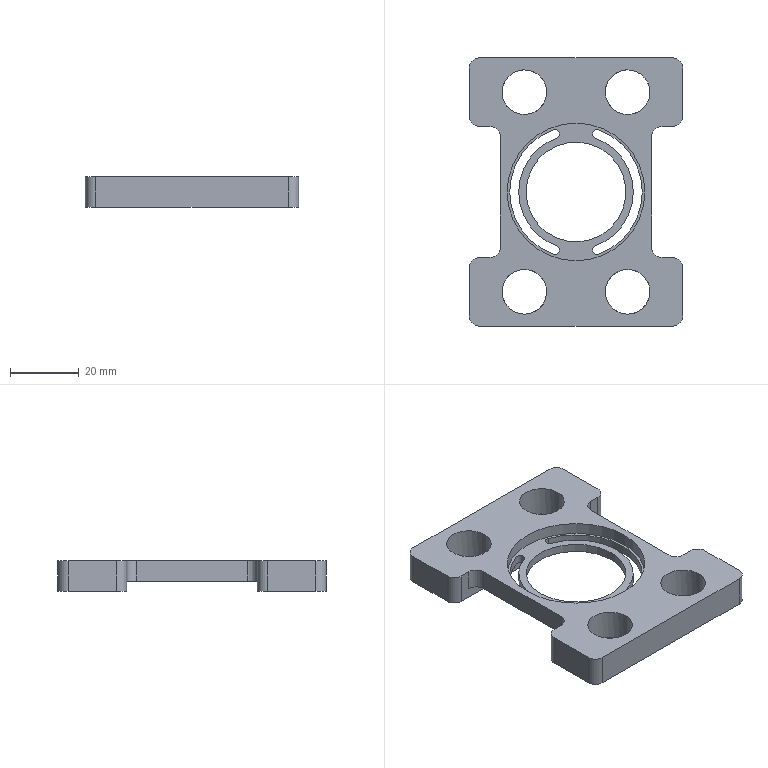NC program | NX | posted with a generic post | part box 62 x 78 x 9 mm
Lines 2826 to 3044 of 3044:
(PLANAR_MILL , TOOL : D6A45)
N5608 T07 M6
N5610 G54
N5612 G17 G0 G90 X-34.243 Y-14.234 S9500 M3
N5614 G43 Z30. H7
N5616 Z0.
N5618 G94 G1 Z-1. F1250.
N5620 G3 X-34.6 Y-15. R1.
N5622 X-29. Y-20.6 R5.6
N5624 X-34.6 Y-15. R-5.6
N5626 X-34.243 Y-15.766 R1.
N5628 G1 Z0.
N5630 G0 Z30.
N5632 Y15.766
N5634 Z0.
N5636 G1 Z-1.
N5638 G3 X-34.6 Y15. R1.
N5640 X-29. Y9.4 R5.6
N5642 X-34.6 Y15. R-5.6
N5644 X-34.243 Y14.234 R1.
N5646 G1 Z0.
N5648 G0 Z30.
N5650 X-40.257 Y-0.766
N5652 Z0.
N5654 G1 Z-1.
N5656 G3 X-39.9 Y0. R1.
N5658 G1 Y28.
N5660 G2 X-36. Y31.9 R3.9
N5662 G1 X-22.
N5664 G2 X-18.1 Y28. R3.9
N5666 G1 Y25.
N5668 G3 X-16. Y22.9 R2.1
N5670 G1 X16.
N5672 G3 X18.1 Y25. R2.1
N5674 G1 Y28.
N5676 G2 X22. Y31.9 R3.9
N5678 G1 X36.
N5680 G2 X39.9 Y28. R3.9
N5682 G1 Y-28.
N5684 G2 X36. Y-31.9 R3.9
N5686 G1 X22.
N5688 G2 X18.1 Y-28. R3.9
N5690 G1 Y-25.
N5692 G3 X16. Y-22.9 R2.1
N5694 G1 X-16.
N5696 G3 X-18.1 Y-25. R2.1
N5698 G1 Y-28.
N5700 G2 X-22. Y-31.9 R3.9
N5702 G1 X-36.
N5704 G2 X-39.9 Y-28. R3.9
N5706 G1 Y0.
N5708 G3 X-40.257 Y0.766 R1.
N5710 G1 Z0.
N5712 G0 Z30.
N5714 X0.766 Y18.743
N5716 Z0.
N5718 G1 Z-1.
N5720 G3 X0. Y19.1 R1.
N5722 X-19.1 Y0. R19.1
N5724 X0. Y19.1 R-19.1
N5726 X-0.766 Y18.743 R1.
N5728 G1 Z0.
N5730 G0 Z30.
N5732 X34.243 Y-15.766
N5734 Z0.
N5736 G1 Z-1.
N5738 G3 X34.6 Y-15. R1.
N5740 X29. Y-9.4 R5.6
N5742 X34.6 Y-15. R-5.6
N5744 X34.243 Y-14.234 R1.
N5746 G1 Z0.
N5748 G0 Z30.
N5750 Y14.234
N5752 Z0.
N5754 G1 Z-1.
N5756 G3 X34.6 Y15. R1.
N5758 X29. Y20.6 R5.6
N5760 X34.6 Y15. R-5.6
N5762 X34.243 Y15.766 R1.
N5764 G1 Z0.
N5766 G0 Z30.
(PLANAR_MILL_COPY , TOOL : D6A45)
N5768 X0.766 Y13.243
N5770 Z-3.5
N5772 G1 Z-4.5
N5774 G3 X0. Y13.6 R1.
N5776 X-13.6 Y0. R13.6
N5778 X0. Y13.6 R-13.6
N5780 X-0.766 Y13.243 R1.
N5782 G1 Z-3.5
N5784 G0 Z30.
N5786 M5
(ZLEVEL_PROFILE_COPY_2 , TOOL : D6)
N5788 T06 M6
N5790 G54
N5792 G17 G0 G90 X-42. Y-23.258 S9500 M3
N5794 G43 Z30. H6
N5796 Z-0.4
N5798 G94 G1 Y28.601 Z-3.118 F1000.
N5800 X-41.613 Y30.203 Z-3.204
N5802 X-40.807 Y31.641 Z-3.291
N5804 X-39.641 Y32.807 Z-3.377
N5806 X-38.203 Y33.613 Z-3.463
N5808 X-36.601 Y34. Z-3.55
N5810 X-21.399 Z-4.346
N5812 X-19.797 Y33.613 Z-4.433
N5814 X-18.359 Y32.807 Z-4.519
N5816 X-17.193 Y31.641 Z-4.606
N5818 X-16.387 Y30.203 Z-4.692
N5820 X-16. Y28.601 Z-4.778
N5822 Y25. Z-4.967
N5824 X16. Z-6.644
N5826 Y28.601 Z-6.833
N5828 X16.387 Y30.203 Z-6.919
N5830 X17.193 Y31.641 Z-7.006
N5832 X18.359 Y32.807 Z-7.092
N5834 X19.797 Y33.613 Z-7.178
N5836 X21.399 Y34. Z-7.265
N5838 X36.601 Z-8.062
N5840 X38.203 Y33.613 Z-8.148
N5842 X39.641 Y32.807 Z-8.234
N5844 X40.807 Y31.641 Z-8.321
N5846 X41.613 Y30.203 Z-8.407
N5848 X42. Y28.601 Z-8.494
N5850 Y28. Z-8.525
N5852 Y-28. F1200.
N5854 G2 X36. Y-34. R6.
N5856 G1 X22.
N5858 G2 X16. Y-28. R6.
N5860 G1 Y-25.
N5862 X-16.
N5864 Y-28.
N5866 G2 X-22. Y-34. R6.
N5868 G1 X-36.
N5870 G2 X-42. Y-28. R6.
N5872 G1 Y28.
N5874 G2 X-36. Y34. R6.
N5876 G1 X-22.
N5878 G2 X-16. Y28. R6.
N5880 G1 Y25.
N5882 X16.
N5884 Y28.
N5886 G2 X22. Y34. R6.
N5888 G1 X36.
N5890 G2 X42. Y28. R6.
N5892 G1 Y20.839 Z-8.65
N5894 Y-28.
N5896 G2 X36. Y-34. R6.
N5898 G1 X22.
N5900 G2 X16. Y-28. R6.
N5902 G1 Y-25.
N5904 X-16.
N5906 Y-28.
N5908 G2 X-22. Y-34. R6.
N5910 G1 X-36.
N5912 G2 X-42. Y-28. R6.
N5914 G1 Y28.
N5916 G2 X-36. Y34. R6.
N5918 G1 X-22.
N5920 G2 X-16. Y28. R6.
N5922 G1 Y25.
N5924 X16.
N5926 Y28.
N5928 G2 X22. Y34. R6.
N5930 G1 X36.
N5932 G2 X42. Y28. R6.
N5934 G1 Y20.839 Z-8.775
N5936 Y-28.
N5938 G2 X36. Y-34. R6.
N5940 G1 X22.
N5942 G2 X16. Y-28. R6.
N5944 G1 Y-25.
N5946 X-16.
N5948 Y-28.
N5950 G2 X-22. Y-34. R6.
N5952 G1 X-36.
N5954 G2 X-42. Y-28. R6.
N5956 G1 Y28.
N5958 G2 X-36. Y34. R6.
N5960 G1 X-22.
N5962 G2 X-16. Y28. R6.
N5964 G1 Y25.
N5966 X16.
N5968 Y28.
N5970 G2 X22. Y34. R6.
N5972 G1 X36.
N5974 G2 X42. Y28. R6.
N5976 G1 Y20.839 Z-8.9
N5978 Y-28.
N5980 G2 X36. Y-34. R6.
N5982 G1 X22.
N5984 G2 X16. Y-28. R6.
N5986 G1 Y-25.
N5988 X-16.
N5990 Y-28.
N5992 G2 X-22. Y-34. R6.
N5994 G1 X-36.
N5996 G2 X-42. Y-28. R6.
N5998 G1 Y28.
N6000 G2 X-36. Y34. R6.
N6002 G1 X-22.
N6004 G2 X-16. Y28. R6.
N6006 G1 Y25.
N6008 X16.
N6010 Y28.
N6012 G2 X22. Y34. R6.
N6014 G1 X36.
N6016 G2 X42. Y28. R6.
N6018 G1 Y20.839
N6020 Z-0.9
N6022 G0 Z30.
N6024 M5
N6026 M2